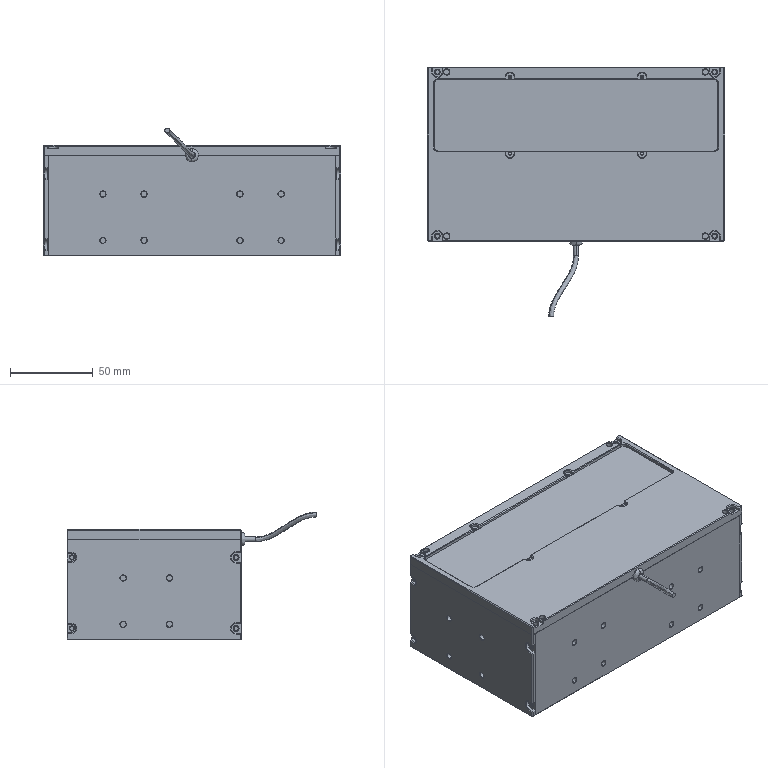Part | SolidWorks | 15 solids | 805 faces | box 180 x 151.4 x 77.5 mm | volume 341470 mm3 | plane 425 | cylinder 216 | cone 158 | spline 6 | commonest cylinder face diameters 3.5 x56 3.2 x26 2.5 x24 1.6 x20 2 x20 2.2 x12